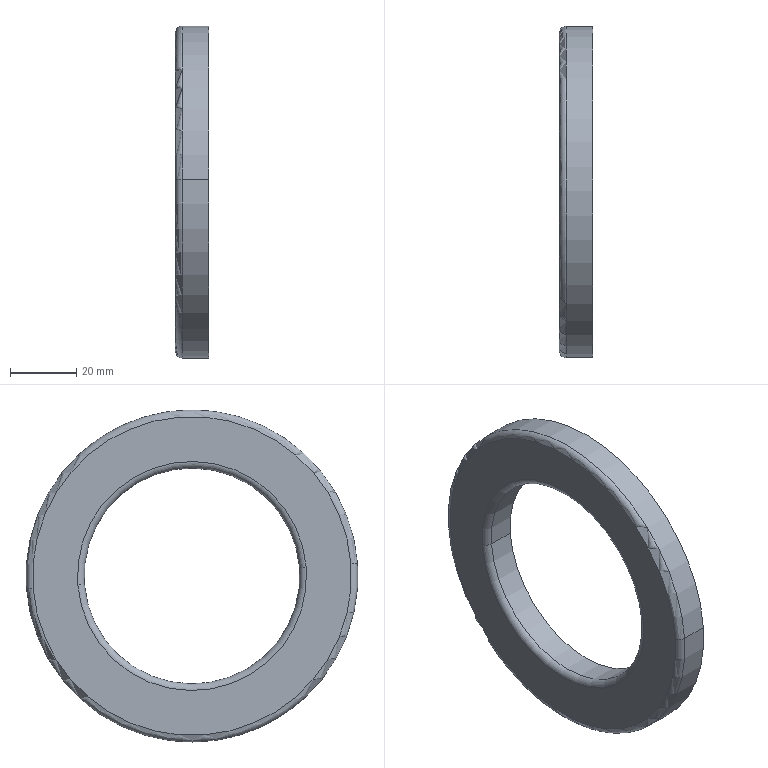Part | STEP file | Input 21 | 1 solid | 20 faces | box 10 x 100 x 100 mm | volume 8867 mm3 | cylinder 8 | torus 8 | plane 4 | commonest cylinder face diameters 65 x2 67 x2 98 x2 100 x2
STEP:
#1=CARTESIAN_POINT('',(0.,0.,0.));
#2=DIRECTION('',(0.,0.,1.));
#3=DIRECTION('',(1.,0.,0.));
#4=AXIS2_PLACEMENT_3D('',#1,#2,#3);
#5=CARTESIAN_POINT('',(-3648.,-33.401,2.578));
#6=VERTEX_POINT('',#5);
#7=CARTESIAN_POINT('',(-3648.,33.401,-2.578));
#8=VERTEX_POINT('',#7);
#9=CARTESIAN_POINT('',(-3648.,0.,0.));
#10=DIRECTION('',(1.,0.,0.));
#11=DIRECTION('',(0.,-0.997,0.07695));
#12=AXIS2_PLACEMENT_3D('',#9,#10,#11);
#13=CIRCLE('',#12,33.5);
#14=CARTESIAN_POINT('',(-3640.,0.,0.));
#15=DIRECTION('',(1.,0.,0.));
#16=DIRECTION('',(0.,-0.997,0.07695));
#17=AXIS2_PLACEMENT_3D('',#14,#15,#16);
#18=CYLINDRICAL_SURFACE('',#17,33.5);
#19=CARTESIAN_POINT('',(0.,-8.));
#20=DIRECTION('',(1.,0.));
#21=VECTOR('',#20,1.);
#22=LINE('',#19,#21);
#23=(GEOMETRIC_REPRESENTATION_CONTEXT(2)PARAMETRIC_REPRESENTATION_CONTEXT()REPRESENTATION_CONTEXT('',''));
#24=DEFINITIONAL_REPRESENTATION('',(#22),#23);
#25=PCURVE('',#18,#24);
#26=CARTESIAN_POINT('',(-3648.,0.,0.));
#27=DIRECTION('',(1.,0.,0.));
#28=DIRECTION('',(0.,-0.997,0.07695));
#29=AXIS2_PLACEMENT_3D('',#26,#27,#28);
#30=TOROIDAL_SURFACE('',#29,34.5,1.);
#31=CARTESIAN_POINT('',(0.,3.142));
#32=DIRECTION('',(1.,0.));
#33=VECTOR('',#32,1.);
#34=LINE('',#31,#33);
#35=(GEOMETRIC_REPRESENTATION_CONTEXT(2)PARAMETRIC_REPRESENTATION_CONTEXT()REPRESENTATION_CONTEXT('',''));
#36=DEFINITIONAL_REPRESENTATION('',(#34),#35);
#37=PCURVE('',#30,#36);
#38=SURFACE_CURVE('',#13,(#25,#37),.PCURVE_S1.);
#39=EDGE_CURVE('',#6,#8,#38,.T.);
#40=ORIENTED_EDGE('',*,*,#39,.T.);
#41=CARTESIAN_POINT('',(-3640.,33.401,-2.578));
#42=VERTEX_POINT('',#41);
#43=CARTESIAN_POINT('',(-3640.,33.401,-2.578));
#44=DIRECTION('',(1.,0.,0.));
#45=VECTOR('',#44,1.);
#46=LINE('',#43,#45);
#47=CARTESIAN_POINT('',(3.142,0.));
#48=DIRECTION('',(0.,1.));
#49=VECTOR('',#48,1.);
#50=LINE('',#47,#49);
#51=(GEOMETRIC_REPRESENTATION_CONTEXT(2)PARAMETRIC_REPRESENTATION_CONTEXT()REPRESENTATION_CONTEXT('',''));
#52=DEFINITIONAL_REPRESENTATION('',(#50),#51);
#53=PCURVE('',#18,#52);
#54=CARTESIAN_POINT('',(-3640.,0.,0.));
#55=DIRECTION('',(1.,0.,0.));
#56=DIRECTION('',(0.,-0.997,0.07695));
#57=AXIS2_PLACEMENT_3D('',#54,#55,#56);
#58=CYLINDRICAL_SURFACE('',#57,33.5);
#59=CARTESIAN_POINT('',(3.142,0.));
#60=DIRECTION('',(0.,1.));
#61=VECTOR('',#60,1.);
#62=LINE('',#59,#61);
#63=(GEOMETRIC_REPRESENTATION_CONTEXT(2)PARAMETRIC_REPRESENTATION_CONTEXT()REPRESENTATION_CONTEXT('',''));
#64=DEFINITIONAL_REPRESENTATION('',(#62),#63);
#65=PCURVE('',#58,#64);
#66=SURFACE_CURVE('',#46,(#53,#65),.PCURVE_S1.);
#67=EDGE_CURVE('',#8,#42,#66,.T.);
#68=ORIENTED_EDGE('',*,*,#67,.T.);
#69=CARTESIAN_POINT('',(-3640.,-33.401,2.578));
#70=VERTEX_POINT('',#69);
#71=CARTESIAN_POINT('',(-3640.,0.,0.));
#72=DIRECTION('',(1.,0.,0.));
#73=DIRECTION('',(0.,-0.997,0.07695));
#74=AXIS2_PLACEMENT_3D('',#71,#72,#73);
#75=CIRCLE('',#74,33.5);
#76=CARTESIAN_POINT('',(0.,0.));
#77=DIRECTION('',(1.,0.));
#78=VECTOR('',#77,1.);
#79=LINE('',#76,#78);
#80=(GEOMETRIC_REPRESENTATION_CONTEXT(2)PARAMETRIC_REPRESENTATION_CONTEXT()REPRESENTATION_CONTEXT('',''));
#81=DEFINITIONAL_REPRESENTATION('',(#79),#80);
#82=PCURVE('',#18,#81);
#83=CARTESIAN_POINT('',(-3640.,-33.401,2.578));
#84=DIRECTION('',(1.,0.,0.));
#85=DIRECTION('',(0.,-0.997,0.07695));
#86=AXIS2_PLACEMENT_3D('',#83,#84,#85);
#87=PLANE('',#86);
#88=CARTESIAN_POINT('',(-33.5,0.));
#89=DIRECTION('',(1.,0.));
#90=AXIS2_PLACEMENT_2D('',#88,#89);
#91=CIRCLE('',#90,33.5);
#92=(GEOMETRIC_REPRESENTATION_CONTEXT(2)PARAMETRIC_REPRESENTATION_CONTEXT()REPRESENTATION_CONTEXT('',''));
#93=DEFINITIONAL_REPRESENTATION('',(#91),#92);
#94=PCURVE('',#87,#93);
#95=SURFACE_CURVE('',#75,(#82,#94),.PCURVE_S1.);
#96=EDGE_CURVE('',#70,#42,#95,.T.);
#97=ORIENTED_EDGE('',*,*,#96,.F.);
#98=CARTESIAN_POINT('',(-3640.,-33.401,2.578));
#99=DIRECTION('',(1.,0.,0.));
#100=VECTOR('',#99,1.);
#101=LINE('',#98,#100);
#102=CARTESIAN_POINT('',(0.,0.));
#103=DIRECTION('',(0.,1.));
#104=VECTOR('',#103,1.);
#105=LINE('',#102,#104);
#106=(GEOMETRIC_REPRESENTATION_CONTEXT(2)PARAMETRIC_REPRESENTATION_CONTEXT()REPRESENTATION_CONTEXT('',''));
#107=DEFINITIONAL_REPRESENTATION('',(#105),#106);
#108=PCURVE('',#18,#107);
#109=CARTESIAN_POINT('',(6.283,0.));
#110=DIRECTION('',(0.,1.));
#111=VECTOR('',#110,1.);
#112=LINE('',#109,#111);
#113=(GEOMETRIC_REPRESENTATION_CONTEXT(2)PARAMETRIC_REPRESENTATION_CONTEXT()REPRESENTATION_CONTEXT('',''));
#114=DEFINITIONAL_REPRESENTATION('',(#112),#113);
#115=PCURVE('',#58,#114);
#116=SURFACE_CURVE('',#101,(#108,#115),.PCURVE_S1.);
#117=EDGE_CURVE('',#6,#70,#116,.T.);
#118=ORIENTED_EDGE('',*,*,#117,.F.);
#119=EDGE_LOOP('',(#40,#68,#97,#118));
#120=FACE_BOUND('',#119,.T.);
#121=ADVANCED_FACE('',(#120),#18,.T.);
#122=CARTESIAN_POINT('',(-3649.,-34.398,2.655));
#123=VERTEX_POINT('',#122);
#124=CARTESIAN_POINT('',(-3648.,-34.398,2.655));
#125=DIRECTION('',(0.,0.07695,0.997));
#126=DIRECTION('',(0.,-0.997,0.07695));
#127=AXIS2_PLACEMENT_3D('',#124,#125,#126);
#128=CIRCLE('',#127,1.);
#129=CARTESIAN_POINT('',(-3648.,0.,0.));
#130=DIRECTION('',(1.,0.,0.));
#131=DIRECTION('',(0.,-0.997,0.07695));
#132=AXIS2_PLACEMENT_3D('',#129,#130,#131);
#133=TOROIDAL_SURFACE('',#132,34.5,1.);
#134=CARTESIAN_POINT('',(6.283,0.));
#135=DIRECTION('',(0.,1.));
#136=VECTOR('',#135,1.);
#137=LINE('',#134,#136);
#138=(GEOMETRIC_REPRESENTATION_CONTEXT(2)PARAMETRIC_REPRESENTATION_CONTEXT()REPRESENTATION_CONTEXT('',''));
#139=DEFINITIONAL_REPRESENTATION('',(#137),#138);
#140=PCURVE('',#133,#139);
#141=CARTESIAN_POINT('',(0.,0.));
#142=DIRECTION('',(0.,1.));
#143=VECTOR('',#142,1.);
#144=LINE('',#141,#143);
#145=(GEOMETRIC_REPRESENTATION_CONTEXT(2)PARAMETRIC_REPRESENTATION_CONTEXT()REPRESENTATION_CONTEXT('',''));
#146=DEFINITIONAL_REPRESENTATION('',(#144),#145);
#147=PCURVE('',#30,#146);
#148=SURFACE_CURVE('',#128,(#140,#147),.PCURVE_S1.);
#149=EDGE_CURVE('',#6,#123,#148,.T.);
#150=ORIENTED_EDGE('',*,*,#149,.T.);
#151=CARTESIAN_POINT('',(-3649.,34.398,-2.655));
#152=VERTEX_POINT('',#151);
#153=CARTESIAN_POINT('',(-3649.,0.,0.));
#154=DIRECTION('',(1.,0.,0.));
#155=DIRECTION('',(0.,-0.997,0.07695));
#156=AXIS2_PLACEMENT_3D('',#153,#154,#155);
#157=CIRCLE('',#156,34.5);
#158=CARTESIAN_POINT('',(0.,4.712));
#159=DIRECTION('',(1.,0.));
#160=VECTOR('',#159,1.);
#161=LINE('',#158,#160);
#162=(GEOMETRIC_REPRESENTATION_CONTEXT(2)PARAMETRIC_REPRESENTATION_CONTEXT()REPRESENTATION_CONTEXT('',''));
#163=DEFINITIONAL_REPRESENTATION('',(#161),#162);
#164=PCURVE('',#133,#163);
#165=CARTESIAN_POINT('',(-3649.,-47.858,3.694));
#166=DIRECTION('',(1.,0.,0.));
#167=DIRECTION('',(0.,-0.997,0.07695));
#168=AXIS2_PLACEMENT_3D('',#165,#166,#167);
#169=PLANE('',#168);
#170=CARTESIAN_POINT('',(-48.,0.));
#171=DIRECTION('',(1.,0.));
#172=AXIS2_PLACEMENT_2D('',#170,#171);
#173=CIRCLE('',#172,34.5);
#174=(GEOMETRIC_REPRESENTATION_CONTEXT(2)PARAMETRIC_REPRESENTATION_CONTEXT()REPRESENTATION_CONTEXT('',''));
#175=DEFINITIONAL_REPRESENTATION('',(#173),#174);
#176=PCURVE('',#169,#175);
#177=SURFACE_CURVE('',#157,(#164,#176),.PCURVE_S1.);
#178=EDGE_CURVE('',#152,#123,#177,.T.);
#179=ORIENTED_EDGE('',*,*,#178,.F.);
#180=CARTESIAN_POINT('',(-3648.,34.398,-2.655));
#181=DIRECTION('',(0.,-0.07695,-0.997));
#182=DIRECTION('',(0.,0.997,-0.07695));
#183=AXIS2_PLACEMENT_3D('',#180,#181,#182);
#184=CIRCLE('',#183,1.);
#185=CARTESIAN_POINT('',(3.142,0.));
#186=DIRECTION('',(0.,1.));
#187=VECTOR('',#186,1.);
#188=LINE('',#185,#187);
#189=(GEOMETRIC_REPRESENTATION_CONTEXT(2)PARAMETRIC_REPRESENTATION_CONTEXT()REPRESENTATION_CONTEXT('',''));
#190=DEFINITIONAL_REPRESENTATION('',(#188),#189);
#191=PCURVE('',#133,#190);
#192=CARTESIAN_POINT('',(3.142,0.));
#193=DIRECTION('',(0.,1.));
#194=VECTOR('',#193,1.);
#195=LINE('',#192,#194);
#196=(GEOMETRIC_REPRESENTATION_CONTEXT(2)PARAMETRIC_REPRESENTATION_CONTEXT()REPRESENTATION_CONTEXT('',''));
#197=DEFINITIONAL_REPRESENTATION('',(#195),#196);
#198=PCURVE('',#30,#197);
#199=SURFACE_CURVE('',#184,(#191,#198),.PCURVE_S1.);
#200=EDGE_CURVE('',#8,#152,#199,.T.);
#201=ORIENTED_EDGE('',*,*,#200,.F.);
#202=CARTESIAN_POINT('',(-3648.,0.,0.));
#203=DIRECTION('',(1.,0.,0.));
#204=DIRECTION('',(0.,-0.997,0.07695));
#205=AXIS2_PLACEMENT_3D('',#202,#203,#204);
#206=CIRCLE('',#205,33.5);
#207=CARTESIAN_POINT('',(0.,3.142));
#208=DIRECTION('',(1.,0.));
#209=VECTOR('',#208,1.);
#210=LINE('',#207,#209);
#211=(GEOMETRIC_REPRESENTATION_CONTEXT(2)PARAMETRIC_REPRESENTATION_CONTEXT()REPRESENTATION_CONTEXT('',''));
#212=DEFINITIONAL_REPRESENTATION('',(#210),#211);
#213=PCURVE('',#133,#212);
#214=CARTESIAN_POINT('',(0.,-8.));
#215=DIRECTION('',(1.,0.));
#216=VECTOR('',#215,1.);
#217=LINE('',#214,#216);
#218=(GEOMETRIC_REPRESENTATION_CONTEXT(2)PARAMETRIC_REPRESENTATION_CONTEXT()REPRESENTATION_CONTEXT('',''));
#219=DEFINITIONAL_REPRESENTATION('',(#217),#218);
#220=PCURVE('',#58,#219);
#221=SURFACE_CURVE('',#206,(#213,#220),.PCURVE_S1.);
#222=EDGE_CURVE('',#8,#6,#221,.T.);
#223=ORIENTED_EDGE('',*,*,#222,.T.);
#224=EDGE_LOOP('',(#150,#179,#201,#223));
#225=FACE_BOUND('',#224,.F.);
#226=ADVANCED_FACE('',(#225),#133,.F.);
#227=CARTESIAN_POINT('',(-3649.,-47.858,3.694));
#228=VERTEX_POINT('',#227);
#229=CARTESIAN_POINT('',(-3648.,-48.855,3.771));
#230=VERTEX_POINT('',#229);
#231=CARTESIAN_POINT('',(-3648.,-47.858,3.694));
#232=DIRECTION('',(0.,0.07695,0.997));
#233=DIRECTION('',(0.,-0.997,0.07695));
#234=AXIS2_PLACEMENT_3D('',#231,#232,#233);
#235=CIRCLE('',#234,1.);
#236=CARTESIAN_POINT('',(-3648.,0.,0.));
#237=DIRECTION('',(1.,0.,0.));
#238=DIRECTION('',(0.,-0.997,0.07695));
#239=AXIS2_PLACEMENT_3D('',#236,#237,#238);
#240=TOROIDAL_SURFACE('',#239,48.,1.);
#241=CARTESIAN_POINT('',(6.283,0.));
#242=DIRECTION('',(0.,1.));
#243=VECTOR('',#242,1.);
#244=LINE('',#241,#243);
#245=(GEOMETRIC_REPRESENTATION_CONTEXT(2)PARAMETRIC_REPRESENTATION_CONTEXT()REPRESENTATION_CONTEXT('',''));
#246=DEFINITIONAL_REPRESENTATION('',(#244),#245);
#247=PCURVE('',#240,#246);
#248=CARTESIAN_POINT('',(-3648.,0.,0.));
#249=DIRECTION('',(1.,0.,0.));
#250=DIRECTION('',(0.,-0.997,0.07695));
#251=AXIS2_PLACEMENT_3D('',#248,#249,#250);
#252=TOROIDAL_SURFACE('',#251,48.,1.);
#253=CARTESIAN_POINT('',(0.,0.));
#254=DIRECTION('',(0.,1.));
#255=VECTOR('',#254,1.);
#256=LINE('',#253,#255);
#257=(GEOMETRIC_REPRESENTATION_CONTEXT(2)PARAMETRIC_REPRESENTATION_CONTEXT()REPRESENTATION_CONTEXT('',''));
#258=DEFINITIONAL_REPRESENTATION('',(#256),#257);
#259=PCURVE('',#252,#258);
#260=SURFACE_CURVE('',#235,(#247,#259),.PCURVE_S1.);
#261=EDGE_CURVE('',#228,#230,#260,.T.);
#262=ORIENTED_EDGE('',*,*,#261,.T.);
#263=CARTESIAN_POINT('',(-3648.,48.855,-3.771));
#264=VERTEX_POINT('',#263);
#265=CARTESIAN_POINT('',(-3648.,0.,0.));
#266=DIRECTION('',(1.,0.,0.));
#267=DIRECTION('',(0.,-0.997,0.07695));
#268=AXIS2_PLACEMENT_3D('',#265,#266,#267);
#269=CIRCLE('',#268,49.);
#270=CARTESIAN_POINT('',(0.,6.283));
#271=DIRECTION('',(1.,0.));
#272=VECTOR('',#271,1.);
#273=LINE('',#270,#272);
#274=(GEOMETRIC_REPRESENTATION_CONTEXT(2)PARAMETRIC_REPRESENTATION_CONTEXT()REPRESENTATION_CONTEXT('',''));
#275=DEFINITIONAL_REPRESENTATION('',(#273),#274);
#276=PCURVE('',#240,#275);
#277=CARTESIAN_POINT('',(-3640.,0.,0.));
#278=DIRECTION('',(1.,0.,0.));
#279=DIRECTION('',(0.,-0.997,0.07695));
#280=AXIS2_PLACEMENT_3D('',#277,#278,#279);
#281=CYLINDRICAL_SURFACE('',#280,49.);
#282=CARTESIAN_POINT('',(0.,-8.));
#283=DIRECTION('',(1.,0.));
#284=VECTOR('',#283,1.);
#285=LINE('',#282,#284);
#286=(GEOMETRIC_REPRESENTATION_CONTEXT(2)PARAMETRIC_REPRESENTATION_CONTEXT()REPRESENTATION_CONTEXT('',''));
#287=DEFINITIONAL_REPRESENTATION('',(#285),#286);
#288=PCURVE('',#281,#287);
#289=SURFACE_CURVE('',#269,(#276,#288),.PCURVE_S1.);
#290=EDGE_CURVE('',#264,#230,#289,.T.);
#291=ORIENTED_EDGE('',*,*,#290,.F.);
#292=CARTESIAN_POINT('',(-3649.,47.858,-3.694));
#293=VERTEX_POINT('',#292);
#294=CARTESIAN_POINT('',(-3648.,47.858,-3.694));
#295=DIRECTION('',(0.,-0.07695,-0.997));
#296=DIRECTION('',(0.,0.997,-0.07695));
#297=AXIS2_PLACEMENT_3D('',#294,#295,#296);
#298=CIRCLE('',#297,1.);
#299=CARTESIAN_POINT('',(3.142,0.));
#300=DIRECTION('',(0.,1.));
#301=VECTOR('',#300,1.);
#302=LINE('',#299,#301);
#303=(GEOMETRIC_REPRESENTATION_CONTEXT(2)PARAMETRIC_REPRESENTATION_CONTEXT()REPRESENTATION_CONTEXT('',''));
#304=DEFINITIONAL_REPRESENTATION('',(#302),#303);
#305=PCURVE('',#240,#304);
#306=CARTESIAN_POINT('',(3.142,0.));
#307=DIRECTION('',(0.,1.));
#308=VECTOR('',#307,1.);
#309=LINE('',#306,#308);
#310=(GEOMETRIC_REPRESENTATION_CONTEXT(2)PARAMETRIC_REPRESENTATION_CONTEXT()REPRESENTATION_CONTEXT('',''));
#311=DEFINITIONAL_REPRESENTATION('',(#309),#310);
#312=PCURVE('',#252,#311);
#313=SURFACE_CURVE('',#298,(#305,#312),.PCURVE_S1.);
#314=EDGE_CURVE('',#293,#264,#313,.T.);
#315=ORIENTED_EDGE('',*,*,#314,.F.);
#316=CARTESIAN_POINT('',(-3649.,0.,0.));
#317=DIRECTION('',(1.,0.,0.));
#318=DIRECTION('',(0.,-0.997,0.07695));
#319=AXIS2_PLACEMENT_3D('',#316,#317,#318);
#320=CIRCLE('',#319,48.);
#321=CARTESIAN_POINT('',(0.,4.712));
#322=DIRECTION('',(1.,0.));
#323=VECTOR('',#322,1.);
#324=LINE('',#321,#323);
#325=(GEOMETRIC_REPRESENTATION_CONTEXT(2)PARAMETRIC_REPRESENTATION_CONTEXT()REPRESENTATION_CONTEXT('',''));
#326=DEFINITIONAL_REPRESENTATION('',(#324),#325);
#327=PCURVE('',#240,#326);
#328=CARTESIAN_POINT('',(-48.,0.));
#329=DIRECTION('',(1.,0.));
#330=AXIS2_PLACEMENT_2D('',#328,#329);
#331=CIRCLE('',#330,48.);
#332=(GEOMETRIC_REPRESENTATION_CONTEXT(2)PARAMETRIC_REPRESENTATION_CONTEXT()REPRESENTATION_CONTEXT('',''));
#333=DEFINITIONAL_REPRESENTATION('',(#331),#332);
#334=PCURVE('',#169,#333);
#335=SURFACE_CURVE('',#320,(#327,#334),.PCURVE_S1.);
#336=EDGE_CURVE('',#293,#228,#335,.T.);
#337=ORIENTED_EDGE('',*,*,#336,.T.);
#338=EDGE_LOOP('',(#262,#291,#315,#337));
#339=FACE_BOUND('',#338,.F.);
#340=ADVANCED_FACE('',(#339),#240,.F.);
#341=CARTESIAN_POINT('',(-3640.,-48.855,3.771));
#342=VERTEX_POINT('',#341);
#343=CARTESIAN_POINT('',(-3640.,-48.855,3.771));
#344=DIRECTION('',(1.,0.,0.));
#345=VECTOR('',#344,1.);
#346=LINE('',#343,#345);
#347=CARTESIAN_POINT('',(6.283,0.));
#348=DIRECTION('',(0.,1.));
#349=VECTOR('',#348,1.);
#350=LINE('',#347,#349);
#351=(GEOMETRIC_REPRESENTATION_CONTEXT(2)PARAMETRIC_REPRESENTATION_CONTEXT()REPRESENTATION_CONTEXT('',''));
#352=DEFINITIONAL_REPRESENTATION('',(#350),#351);
#353=PCURVE('',#281,#352);
#354=CARTESIAN_POINT('',(-3640.,0.,0.));
#355=DIRECTION('',(1.,0.,0.));
#356=DIRECTION('',(0.,-0.997,0.07695));
#357=AXIS2_PLACEMENT_3D('',#354,#355,#356);
#358=CYLINDRICAL_SURFACE('',#357,49.);
#359=CARTESIAN_POINT('',(0.,0.));
#360=DIRECTION('',(0.,1.));
#361=VECTOR('',#360,1.);
#362=LINE('',#359,#361);
#363=(GEOMETRIC_REPRESENTATION_CONTEXT(2)PARAMETRIC_REPRESENTATION_CONTEXT()REPRESENTATION_CONTEXT('',''));
#364=DEFINITIONAL_REPRESENTATION('',(#362),#363);
#365=PCURVE('',#358,#364);
#366=SURFACE_CURVE('',#346,(#353,#365),.PCURVE_S1.);
#367=EDGE_CURVE('',#230,#342,#366,.T.);
#368=ORIENTED_EDGE('',*,*,#367,.T.);
#369=CARTESIAN_POINT('',(-3640.,48.855,-3.771));
#370=VERTEX_POINT('',#369);
#371=CARTESIAN_POINT('',(-3640.,0.,0.));
#372=DIRECTION('',(1.,0.,0.));
#373=DIRECTION('',(0.,-0.997,0.07695));
#374=AXIS2_PLACEMENT_3D('',#371,#372,#373);
#375=CIRCLE('',#374,49.);
#376=CARTESIAN_POINT('',(0.,0.));
#377=DIRECTION('',(1.,0.));
#378=VECTOR('',#377,1.);
#379=LINE('',#376,#378);
#380=(GEOMETRIC_REPRESENTATION_CONTEXT(2)PARAMETRIC_REPRESENTATION_CONTEXT()REPRESENTATION_CONTEXT('',''));
#381=DEFINITIONAL_REPRESENTATION('',(#379),#380);
#382=PCURVE('',#281,#381);
#383=CARTESIAN_POINT('',(-3640.,-49.852,3.848));
#384=DIRECTION('',(1.,0.,0.));
#385=DIRECTION('',(0.,-0.997,0.07695));
#386=AXIS2_PLACEMENT_3D('',#383,#384,#385);
#387=PLANE('',#386);
#388=CARTESIAN_POINT('',(-50.,0.));
#389=DIRECTION('',(1.,0.));
#390=AXIS2_PLACEMENT_2D('',#388,#389);
#391=CIRCLE('',#390,49.);
#392=(GEOMETRIC_REPRESENTATION_CONTEXT(2)PARAMETRIC_REPRESENTATION_CONTEXT()REPRESENTATION_CONTEXT('',''));
#393=DEFINITIONAL_REPRESENTATION('',(#391),#392);
#394=PCURVE('',#387,#393);
#395=SURFACE_CURVE('',#375,(#382,#394),.PCURVE_S1.);
#396=EDGE_CURVE('',#370,#342,#395,.T.);
#397=ORIENTED_EDGE('',*,*,#396,.F.);
#398=CARTESIAN_POINT('',(-3640.,48.855,-3.771));
#399=DIRECTION('',(1.,0.,0.));
#400=VECTOR('',#399,1.);
#401=LINE('',#398,#400);
#402=CARTESIAN_POINT('',(3.142,0.));
#403=DIRECTION('',(0.,1.));
#404=VECTOR('',#403,1.);
#405=LINE('',#402,#404);
#406=(GEOMETRIC_REPRESENTATION_CONTEXT(2)PARAMETRIC_REPRESENTATION_CONTEXT()REPRESENTATION_CONTEXT('',''));
#407=DEFINITIONAL_REPRESENTATION('',(#405),#406);
#408=PCURVE('',#281,#407);
#409=CARTESIAN_POINT('',(3.142,0.));
#410=DIRECTION('',(0.,1.));
#411=VECTOR('',#410,1.);
#412=LINE('',#409,#411);
#413=(GEOMETRIC_REPRESENTATION_CONTEXT(2)PARAMETRIC_REPRESENTATION_CONTEXT()REPRESENTATION_CONTEXT('',''));
#414=DEFINITIONAL_REPRESENTATION('',(#412),#413);
#415=PCURVE('',#358,#414);
#416=SURFACE_CURVE('',#401,(#408,#415),.PCURVE_S1.);
#417=EDGE_CURVE('',#264,#370,#416,.T.);
#418=ORIENTED_EDGE('',*,*,#417,.F.);
#419=ORIENTED_EDGE('',*,*,#290,.T.);
#420=EDGE_LOOP('',(#368,#397,#418,#419));
#421=FACE_BOUND('',#420,.F.);
#422=ADVANCED_FACE('',(#421),#281,.F.);
#423=CARTESIAN_POINT('',(-3648.,-49.852,3.848));
#424=VERTEX_POINT('',#423);
#425=CARTESIAN_POINT('',(-3648.,49.852,-3.848));
#426=VERTEX_POINT('',#425);
#427=CARTESIAN_POINT('',(-3648.,0.,0.));
#428=DIRECTION('',(1.,0.,0.));
#429=DIRECTION('',(0.,-0.997,0.07695));
#430=AXIS2_PLACEMENT_3D('',#427,#428,#429);
#431=CIRCLE('',#430,50.);
#432=CARTESIAN_POINT('',(-3640.,0.,0.));
#433=DIRECTION('',(1.,0.,0.));
#434=DIRECTION('',(0.,-0.997,0.07695));
#435=AXIS2_PLACEMENT_3D('',#432,#433,#434);
#436=CYLINDRICAL_SURFACE('',#435,50.);
#437=CARTESIAN_POINT('',(0.,-8.));
#438=DIRECTION('',(1.,0.));
#439=VECTOR('',#438,1.);
#440=LINE('',#437,#439);
#441=(GEOMETRIC_REPRESENTATION_CONTEXT(2)PARAMETRIC_REPRESENTATION_CONTEXT()REPRESENTATION_CONTEXT('',''));
#442=DEFINITIONAL_REPRESENTATION('',(#440),#441);
#443=PCURVE('',#436,#442);
#444=CARTESIAN_POINT('',(-3648.,0.,0.));
#445=DIRECTION('',(1.,0.,0.));
#446=DIRECTION('',(0.,-0.997,0.07695));
#447=AXIS2_PLACEMENT_3D('',#444,#445,#446);
#448=TOROIDAL_SURFACE('',#447,48.,2.);
#449=CARTESIAN_POINT('',(0.,6.283));
#450=DIRECTION('',(1.,0.));
#451=VECTOR('',#450,1.);
#452=LINE('',#449,#451);
#453=(GEOMETRIC_REPRESENTATION_CONTEXT(2)PARAMETRIC_REPRESENTATION_CONTEXT()REPRESENTATION_CONTEXT('',''));
#454=DEFINITIONAL_REPRESENTATION('',(#452),#453);
#455=PCURVE('',#448,#454);
#456=SURFACE_CURVE('',#431,(#443,#455),.PCURVE_S1.);
#457=EDGE_CURVE('',#424,#426,#456,.T.);
#458=ORIENTED_EDGE('',*,*,#457,.T.);
#459=CARTESIAN_POINT('',(-3640.,49.852,-3.848));
#460=VERTEX_POINT('',#459);
#461=CARTESIAN_POINT('',(-3640.,49.852,-3.848));
#462=DIRECTION('',(1.,0.,0.));
#463=VECTOR('',#462,1.);
#464=LINE('',#461,#463);
#465=CARTESIAN_POINT('',(3.142,0.));
#466=DIRECTION('',(0.,1.));
#467=VECTOR('',#466,1.);
#468=LINE('',#465,#467);
#469=(GEOMETRIC_REPRESENTATION_CONTEXT(2)PARAMETRIC_REPRESENTATION_CONTEXT()REPRESENTATION_CONTEXT('',''));
#470=DEFINITIONAL_REPRESENTATION('',(#468),#469);
#471=PCURVE('',#436,#470);
#472=CARTESIAN_POINT('',(-3640.,0.,0.));
#473=DIRECTION('',(1.,0.,0.));
#474=DIRECTION('',(0.,-0.997,0.07695));
#475=AXIS2_PLACEMENT_3D('',#472,#473,#474);
#476=CYLINDRICAL_SURFACE('',#475,50.);
#477=CARTESIAN_POINT('',(3.142,0.));
#478=DIRECTION('',(0.,1.));
#479=VECTOR('',#478,1.);
#480=LINE('',#477,#479);
#481=(GEOMETRIC_REPRESENTATION_CONTEXT(2)PARAMETRIC_REPRESENTATION_CONTEXT()REPRESENTATION_CONTEXT('',''));
#482=DEFINITIONAL_REPRESENTATION('',(#480),#481);
#483=PCURVE('',#476,#482);
#484=SURFACE_CURVE('',#464,(#471,#483),.PCURVE_S1.);
#485=EDGE_CURVE('',#426,#460,#484,.T.);
#486=ORIENTED_EDGE('',*,*,#485,.T.);
#487=CARTESIAN_POINT('',(-3640.,-49.852,3.848));
#488=VERTEX_POINT('',#487);
#489=CARTESIAN_POINT('',(-3640.,0.,0.));
#490=DIRECTION('',(1.,0.,0.));
#491=DIRECTION('',(0.,-0.997,0.07695));
#492=AXIS2_PLACEMENT_3D('',#489,#490,#491);
#493=CIRCLE('',#492,50.);
#494=CARTESIAN_POINT('',(0.,0.));
#495=DIRECTION('',(1.,0.));
#496=VECTOR('',#495,1.);
#497=LINE('',#494,#496);
#498=(GEOMETRIC_REPRESENTATION_CONTEXT(2)PARAMETRIC_REPRESENTATION_CONTEXT()REPRESENTATION_CONTEXT('',''));
#499=DEFINITIONAL_REPRESENTATION('',(#497),#498);
#500=PCURVE('',#436,#499);
#501=CARTESIAN_POINT('',(-50.,0.));
#502=DIRECTION('',(1.,0.));
#503=AXIS2_PLACEMENT_2D('',#501,#502);
#504=CIRCLE('',#503,50.);
#505=(GEOMETRIC_REPRESENTATION_CONTEXT(2)PARAMETRIC_REPRESENTATION_CONTEXT()REPRESENTATION_CONTEXT('',''));
#506=DEFINITIONAL_REPRESENTATION('',(#504),#505);
#507=PCURVE('',#387,#506);
#508=SURFACE_CURVE('',#493,(#500,#507),.PCURVE_S1.);
#509=EDGE_CURVE('',#488,#460,#508,.T.);
#510=ORIENTED_EDGE('',*,*,#509,.F.);
#511=CARTESIAN_POINT('',(-3640.,-49.852,3.848));
#512=DIRECTION('',(1.,0.,0.));
#513=VECTOR('',#512,1.);
#514=LINE('',#511,#513);
#515=CARTESIAN_POINT('',(0.,0.));
#516=DIRECTION('',(0.,1.));
#517=VECTOR('',#516,1.);
#518=LINE('',#515,#517);
#519=(GEOMETRIC_REPRESENTATION_CONTEXT(2)PARAMETRIC_REPRESENTATION_CONTEXT()REPRESENTATION_CONTEXT('',''));
#520=DEFINITIONAL_REPRESENTATION('',(#518),#519);
#521=PCURVE('',#436,#520);
#522=CARTESIAN_POINT('',(6.283,0.));
#523=DIRECTION('',(0.,1.));
#524=VECTOR('',#523,1.);
#525=LINE('',#522,#524);
#526=(GEOMETRIC_REPRESENTATION_CONTEXT(2)PARAMETRIC_REPRESENTATION_CONTEXT()REPRESENTATION_CONTEXT('',''));
#527=DEFINITIONAL_REPRESENTATION('',(#525),#526);
#528=PCURVE('',#476,#527);
#529=SURFACE_CURVE('',#514,(#521,#528),.PCURVE_S1.);
#530=EDGE_CURVE('',#424,#488,#529,.T.);
#531=ORIENTED_EDGE('',*,*,#530,.F.);
#532=EDGE_LOOP('',(#458,#486,#510,#531));
#533=FACE_BOUND('',#532,.T.);
#534=ADVANCED_FACE('',(#533),#436,.T.);
#535=CARTESIAN_POINT('',(-3650.,-47.858,3.694));
#536=VERTEX_POINT('',#535);
#537=CARTESIAN_POINT('',(-3650.,47.858,-3.694));
#538=VERTEX_POINT('',#537);
#539=CARTESIAN_POINT('',(-3650.,0.,0.));
#540=DIRECTION('',(1.,0.,0.));
#541=DIRECTION('',(0.,-0.997,0.07695));
#542=AXIS2_PLACEMENT_3D('',#539,#540,#541);
#543=CIRCLE('',#542,48.);
#544=CARTESIAN_POINT('',(0.,4.712));
#545=DIRECTION('',(1.,0.));
#546=VECTOR('',#545,1.);
#547=LINE('',#544,#546);
#548=(GEOMETRIC_REPRESENTATION_CONTEXT(2)PARAMETRIC_REPRESENTATION_CONTEXT()REPRESENTATION_CONTEXT('',''));
#549=DEFINITIONAL_REPRESENTATION('',(#547),#548);
#550=PCURVE('',#448,#549);
#551=CARTESIAN_POINT('',(-3650.,-34.398,2.655));
#552=DIRECTION('',(-1.,0.,0.));
#553=DIRECTION('',(0.,0.997,-0.07695));
#554=AXIS2_PLACEMENT_3D('',#551,#552,#553);
#555=PLANE('',#554);
#556=CARTESIAN_POINT('',(-13.5,0.));
#557=CARTESIAN_POINT('',(-13.5,83.138));
#558=CARTESIAN_POINT('',(58.5,41.569));
#559=CARTESIAN_POINT('',(130.5,0.));
#560=CARTESIAN_POINT('',(58.5,-41.569));
#561=CARTESIAN_POINT('',(-13.5,-83.138));
#562=CARTESIAN_POINT('',(-13.5,0.));
#563=(BOUNDED_CURVE()B_SPLINE_CURVE(2,(#556,#557,#558,#559,#560,#561,#562),.UNSPECIFIED.,.T.,.F.)B_SPLINE_CURVE_WITH_KNOTS((1,2,2,2,2,1),(-2.094,0.,2.094,4.189,6.283,8.378),.UNSPECIFIED.)CURVE()GEOMETRIC_REPRESENTATION_ITEM()RATIONAL_B_SPLINE_CURVE((1.,0.5,1.,0.5,1.,0.5,1.))REPRESENTATION_ITEM(''));
#564=(GEOMETRIC_REPRESENTATION_CONTEXT(2)PARAMETRIC_REPRESENTATION_CONTEXT()REPRESENTATION_CONTEXT('',''));
#565=DEFINITIONAL_REPRESENTATION('',(#563),#564);
#566=PCURVE('',#555,#565);
#567=SURFACE_CURVE('',#543,(#550,#566),.PCURVE_S1.);
#568=EDGE_CURVE('',#536,#538,#567,.T.);
#569=ORIENTED_EDGE('',*,*,#568,.T.);
#570=CARTESIAN_POINT('',(-3648.,47.858,-3.694));
#571=DIRECTION('',(0.,-0.07695,-0.997));
#572=DIRECTION('',(0.,0.997,-0.07695));
#573=AXIS2_PLACEMENT_3D('',#570,#571,#572);
#574=CIRCLE('',#573,2.);
#575=CARTESIAN_POINT('',(3.142,0.));
#576=DIRECTION('',(0.,1.));
#577=VECTOR('',#576,1.);
#578=LINE('',#575,#577);
#579=(GEOMETRIC_REPRESENTATION_CONTEXT(2)PARAMETRIC_REPRESENTATION_CONTEXT()REPRESENTATION_CONTEXT('',''));
#580=DEFINITIONAL_REPRESENTATION('',(#578),#579);
#581=PCURVE('',#448,#580);
#582=CARTESIAN_POINT('',(-3648.,0.,0.));
#583=DIRECTION('',(1.,0.,0.));
#584=DIRECTION('',(0.,-0.997,0.07695));
#585=AXIS2_PLACEMENT_3D('',#582,#583,#584);
#586=TOROIDAL_SURFACE('',#585,48.,2.);
#587=CARTESIAN_POINT('',(3.142,0.));
#588=DIRECTION('',(0.,1.));
#589=VECTOR('',#588,1.);
#590=LINE('',#587,#589);
#591=(GEOMETRIC_REPRESENTATION_CONTEXT(2)PARAMETRIC_REPRESENTATION_CONTEXT()REPRESENTATION_CONTEXT('',''));
#592=DEFINITIONAL_REPRESENTATION('',(#590),#591);
#593=PCURVE('',#586,#592);
#594=SURFACE_CURVE('',#574,(#581,#593),.PCURVE_S1.);
#595=EDGE_CURVE('',#538,#426,#594,.T.);
#596=ORIENTED_EDGE('',*,*,#595,.T.);
#597=ORIENTED_EDGE('',*,*,#457,.F.);
#598=CARTESIAN_POINT('',(-3648.,-47.858,3.694));
#599=DIRECTION('',(0.,0.07695,0.997));
#600=DIRECTION('',(0.,-0.997,0.07695));
#601=AXIS2_PLACEMENT_3D('',#598,#599,#600);
#602=CIRCLE('',#601,2.);
#603=CARTESIAN_POINT('',(0.,0.));
#604=DIRECTION('',(0.,1.));
#605=VECTOR('',#604,1.);
#606=LINE('',#603,#605);
#607=(GEOMETRIC_REPRESENTATION_CONTEXT(2)PARAMETRIC_REPRESENTATION_CONTEXT()REPRESENTATION_CONTEXT('',''));
#608=DEFINITIONAL_REPRESENTATION('',(#606),#607);
#609=PCURVE('',#448,#608);
#610=CARTESIAN_POINT('',(6.283,0.));
#611=DIRECTION('',(0.,1.));
#612=VECTOR('',#611,1.);
#613=LINE('',#610,#612);
#614=(GEOMETRIC_REPRESENTATION_CONTEXT(2)PARAMETRIC_REPRESENTATION_CONTEXT()REPRESENTATION_CONTEXT('',''));
#615=DEFINITIONAL_REPRESENTATION('',(#613),#614);
#616=PCURVE('',#586,#615);
#617=SURFACE_CURVE('',#602,(#609,#616),.PCURVE_S1.);
#618=EDGE_CURVE('',#536,#424,#617,.T.);
#619=ORIENTED_EDGE('',*,*,#618,.F.);
#620=EDGE_LOOP('',(#569,#596,#597,#619));
#621=FACE_BOUND('',#620,.T.);
#622=ADVANCED_FACE('',(#621),#448,.T.);
#623=CARTESIAN_POINT('',(-3648.,-32.404,2.501));
#624=VERTEX_POINT('',#623);
#625=CARTESIAN_POINT('',(-3648.,32.404,-2.501));
#626=VERTEX_POINT('',#625);
#627=CARTESIAN_POINT('',(-3648.,0.,0.));
#628=DIRECTION('',(1.,0.,0.));
#629=DIRECTION('',(0.,-0.997,0.07695));
#630=AXIS2_PLACEMENT_3D('',#627,#628,#629);
#631=CIRCLE('',#630,32.5);
#632=CARTESIAN_POINT('',(-3648.,0.,0.));
#633=DIRECTION('',(1.,0.,0.));
#634=DIRECTION('',(0.,-0.997,0.07695));
#635=AXIS2_PLACEMENT_3D('',#632,#633,#634);
#636=TOROIDAL_SURFACE('',#635,34.5,2.);
#637=CARTESIAN_POINT('',(0.,3.142));
#638=DIRECTION('',(1.,0.));
#639=VECTOR('',#638,1.);
#640=LINE('',#637,#639);
#641=(GEOMETRIC_REPRESENTATION_CONTEXT(2)PARAMETRIC_REPRESENTATION_CONTEXT()REPRESENTATION_CONTEXT('',''));
#642=DEFINITIONAL_REPRESENTATION('',(#640),#641);
#643=PCURVE('',#636,#642);
#644=CARTESIAN_POINT('',(-3640.,0.,0.));
#645=DIRECTION('',(1.,0.,0.));
#646=DIRECTION('',(0.,-0.997,0.07695));
#647=AXIS2_PLACEMENT_3D('',#644,#645,#646);
#648=CYLINDRICAL_SURFACE('',#647,32.5);
#649=CARTESIAN_POINT('',(0.,-8.));
#650=DIRECTION('',(1.,0.));
#651=VECTOR('',#650,1.);
#652=LINE('',#649,#651);
#653=(GEOMETRIC_REPRESENTATION_CONTEXT(2)PARAMETRIC_REPRESENTATION_CONTEXT()REPRESENTATION_CONTEXT('',''));
#654=DEFINITIONAL_REPRESENTATION('',(#652),#653);
#655=PCURVE('',#648,#654);
#656=SURFACE_CURVE('',#631,(#643,#655),.PCURVE_S1.);
#657=EDGE_CURVE('',#624,#626,#656,.T.);
#658=ORIENTED_EDGE('',*,*,#657,.T.);
#659=CARTESIAN_POINT('',(-3650.,34.398,-2.655));
#660=VERTEX_POINT('',#659);
#661=CARTESIAN_POINT('',(-3648.,34.398,-2.655));
#662=DIRECTION('',(0.,-0.07695,-0.997));
#663=DIRECTION('',(0.,0.997,-0.07695));
#664=AXIS2_PLACEMENT_3D('',#661,#662,#663);
#665=CIRCLE('',#664,2.);
#666=CARTESIAN_POINT('',(3.142,0.));
#667=DIRECTION('',(0.,1.));
#668=VECTOR('',#667,1.);
#669=LINE('',#666,#668);
#670=(GEOMETRIC_REPRESENTATION_CONTEXT(2)PARAMETRIC_REPRESENTATION_CONTEXT()REPRESENTATION_CONTEXT('',''));
#671=DEFINITIONAL_REPRESENTATION('',(#669),#670);
#672=PCURVE('',#636,#671);
#673=CARTESIAN_POINT('',(-3648.,0.,0.));
#674=DIRECTION('',(1.,0.,0.));
#675=DIRECTION('',(0.,-0.997,0.07695));
#676=AXIS2_PLACEMENT_3D('',#673,#674,#675);
#677=TOROIDAL_SURFACE('',#676,34.5,2.);
#678=CARTESIAN_POINT('',(3.142,0.));
#679=DIRECTION('',(0.,1.));
#680=VECTOR('',#679,1.);
#681=LINE('',#678,#680);
#682=(GEOMETRIC_REPRESENTATION_CONTEXT(2)PARAMETRIC_REPRESENTATION_CONTEXT()REPRESENTATION_CONTEXT('',''));
#683=DEFINITIONAL_REPRESENTATION('',(#681),#682);
#684=PCURVE('',#677,#683);
#685=SURFACE_CURVE('',#665,(#672,#684),.PCURVE_S1.);
#686=EDGE_CURVE('',#626,#660,#685,.T.);
#687=ORIENTED_EDGE('',*,*,#686,.T.);
#688=CARTESIAN_POINT('',(-3650.,-34.398,2.655));
#689=VERTEX_POINT('',#688);
#690=CARTESIAN_POINT('',(-3650.,0.,0.));
#691=DIRECTION('',(1.,0.,0.));
#692=DIRECTION('',(0.,-0.997,0.07695));
#693=AXIS2_PLACEMENT_3D('',#690,#691,#692);
#694=CIRCLE('',#693,34.5);
#695=CARTESIAN_POINT('',(0.,4.712));
#696=DIRECTION('',(1.,0.));
#697=VECTOR('',#696,1.);
#698=LINE('',#695,#697);
#699=(GEOMETRIC_REPRESENTATION_CONTEXT(2)PARAMETRIC_REPRESENTATION_CONTEXT()REPRESENTATION_CONTEXT('',''));
#700=DEFINITIONAL_REPRESENTATION('',(#698),#699);
#701=PCURVE('',#636,#700);
#702=CARTESIAN_POINT('',(0.,0.));
#703=CARTESIAN_POINT('',(0.,59.756));
#704=CARTESIAN_POINT('',(51.75,29.878));
#705=CARTESIAN_POINT('',(103.5,0.));
#706=CARTESIAN_POINT('',(51.75,-29.878));
#707=CARTESIAN_POINT('',(0.,-59.756));
#708=CARTESIAN_POINT('',(0.,0.));
#709=(BOUNDED_CURVE()B_SPLINE_CURVE(2,(#702,#703,#704,#705,#706,#707,#708),.UNSPECIFIED.,.T.,.F.)B_SPLINE_CURVE_WITH_KNOTS((1,2,2,2,2,1),(-2.094,0.,2.094,4.189,6.283,8.378),.UNSPECIFIED.)CURVE()GEOMETRIC_REPRESENTATION_ITEM()RATIONAL_B_SPLINE_CURVE((1.,0.5,1.,0.5,1.,0.5,1.))REPRESENTATION_ITEM(''));
#710=(GEOMETRIC_REPRESENTATION_CONTEXT(2)PARAMETRIC_REPRESENTATION_CONTEXT()REPRESENTATION_CONTEXT('',''));
#711=DEFINITIONAL_REPRESENTATION('',(#709),#710);
#712=PCURVE('',#555,#711);
#713=SURFACE_CURVE('',#694,(#701,#712),.PCURVE_S1.);
#714=EDGE_CURVE('',#689,#660,#713,.T.);
#715=ORIENTED_EDGE('',*,*,#714,.F.);
#716=CARTESIAN_POINT('',(-3648.,-34.398,2.655));
#717=DIRECTION('',(0.,0.07695,0.997));
#718=DIRECTION('',(0.,-0.997,0.07695));
#719=AXIS2_PLACEMENT_3D('',#716,#717,#718);
#720=CIRCLE('',#719,2.);
#721=CARTESIAN_POINT('',(0.,0.));
#722=DIRECTION('',(0.,1.));
#723=VECTOR('',#722,1.);
#724=LINE('',#721,#723);
#725=(GEOMETRIC_REPRESENTATION_CONTEXT(2)PARAMETRIC_REPRESENTATION_CONTEXT()REPRESENTATION_CONTEXT('',''));
#726=DEFINITIONAL_REPRESENTATION('',(#724),#725);
#727=PCURVE('',#636,#726);
#728=CARTESIAN_POINT('',(6.283,0.));
#729=DIRECTION('',(0.,1.));
#730=VECTOR('',#729,1.);
#731=LINE('',#728,#730);
#732=(GEOMETRIC_REPRESENTATION_CONTEXT(2)PARAMETRIC_REPRESENTATION_CONTEXT()REPRESENTATION_CONTEXT('',''));
#733=DEFINITIONAL_REPRESENTATION('',(#731),#732);
#734=PCURVE('',#677,#733);
#735=SURFACE_CURVE('',#720,(#727,#734),.PCURVE_S1.);
#736=EDGE_CURVE('',#624,#689,#735,.T.);
#737=ORIENTED_EDGE('',*,*,#736,.F.);
#738=EDGE_LOOP('',(#658,#687,#715,#737));
#739=FACE_BOUND('',#738,.T.);
#740=ADVANCED_FACE('',(#739),#636,.T.);
#741=CARTESIAN_POINT('',(-3640.,-32.404,2.501));
#742=VERTEX_POINT('',#741);
#743=CARTESIAN_POINT('',(-3640.,-32.404,2.501));
#744=DIRECTION('',(1.,0.,0.));
#745=VECTOR('',#744,1.);
#746=LINE('',#743,#745);
#747=CARTESIAN_POINT('',(-3640.,0.,0.));
#748=DIRECTION('',(1.,0.,0.));
#749=DIRECTION('',(0.,-0.997,0.07695));
#750=AXIS2_PLACEMENT_3D('',#747,#748,#749);
#751=CYLINDRICAL_SURFACE('',#750,32.5);
#752=CARTESIAN_POINT('',(6.283,0.));
#753=DIRECTION('',(0.,1.));
#754=VECTOR('',#753,1.);
#755=LINE('',#752,#754);
#756=(GEOMETRIC_REPRESENTATION_CONTEXT(2)PARAMETRIC_REPRESENTATION_CONTEXT()REPRESENTATION_CONTEXT('',''));
#757=DEFINITIONAL_REPRESENTATION('',(#755),#756);
#758=PCURVE('',#751,#757);
#759=CARTESIAN_POINT('',(0.,0.));
#760=DIRECTION('',(0.,1.));
#761=VECTOR('',#760,1.);
#762=LINE('',#759,#761);
#763=(GEOMETRIC_REPRESENTATION_CONTEXT(2)PARAMETRIC_REPRESENTATION_CONTEXT()REPRESENTATION_CONTEXT('',''));
#764=DEFINITIONAL_REPRESENTATION('',(#762),#763);
#765=PCURVE('',#648,#764);
#766=SURFACE_CURVE('',#746,(#758,#765),.PCURVE_S1.);
#767=EDGE_CURVE('',#624,#742,#766,.T.);
#768=ORIENTED_EDGE('',*,*,#767,.T.);
#769=CARTESIAN_POINT('',(-3640.,32.404,-2.501));
#770=VERTEX_POINT('',#769);
#771=CARTESIAN_POINT('',(-3640.,0.,0.));
#772=DIRECTION('',(1.,0.,0.));
#773=DIRECTION('',(0.,-0.997,0.07695));
#774=AXIS2_PLACEMENT_3D('',#771,#772,#773);
#775=CIRCLE('',#774,32.5);
#776=CARTESIAN_POINT('',(0.,0.));
#777=DIRECTION('',(1.,0.));
#778=VECTOR('',#777,1.);
#779=LINE('',#776,#778);
#780=(GEOMETRIC_REPRESENTATION_CONTEXT(2)PARAMETRIC_REPRESENTATION_CONTEXT()REPRESENTATION_CONTEXT('',''));
#781=DEFINITIONAL_REPRESENTATION('',(#779),#780);
#782=PCURVE('',#751,#781);
#783=CARTESIAN_POINT('',(-33.5,0.));
#784=DIRECTION('',(1.,0.));
#785=AXIS2_PLACEMENT_2D('',#783,#784);
#786=CIRCLE('',#785,32.5);
#787=(GEOMETRIC_REPRESENTATION_CONTEXT(2)PARAMETRIC_REPRESENTATION_CONTEXT()REPRESENTATION_CONTEXT('',''));
#788=DEFINITIONAL_REPRESENTATION('',(#786),#787);
#789=PCURVE('',#87,#788);
#790=SURFACE_CURVE('',#775,(#782,#789),.PCURVE_S1.);
#791=EDGE_CURVE('',#770,#742,#790,.T.);
#792=ORIENTED_EDGE('',*,*,#791,.F.);
#793=CARTESIAN_POINT('',(-3640.,32.404,-2.501));
#794=DIRECTION('',(1.,0.,0.));
#795=VECTOR('',#794,1.);
#796=LINE('',#793,#795);
#797=CARTESIAN_POINT('',(3.142,0.));
#798=DIRECTION('',(0.,1.));
#799=VECTOR('',#798,1.);
#800=LINE('',#797,#799);
#801=(GEOMETRIC_REPRESENTATION_CONTEXT(2)PARAMETRIC_REPRESENTATION_CONTEXT()REPRESENTATION_CONTEXT('',''));
#802=DEFINITIONAL_REPRESENTATION('',(#800),#801);
#803=PCURVE('',#751,#802);
#804=CARTESIAN_POINT('',(3.142,0.));
#805=DIRECTION('',(0.,1.));
#806=VECTOR('',#805,1.);
#807=LINE('',#804,#806);
#808=(GEOMETRIC_REPRESENTATION_CONTEXT(2)PARAMETRIC_REPRESENTATION_CONTEXT()REPRESENTATION_CONTEXT('',''));
#809=DEFINITIONAL_REPRESENTATION('',(#807),#808);
#810=PCURVE('',#648,#809);
#811=SURFACE_CURVE('',#796,(#803,#810),.PCURVE_S1.);
#812=EDGE_CURVE('',#626,#770,#811,.T.);
#813=ORIENTED_EDGE('',*,*,#812,.F.);
#814=CARTESIAN_POINT('',(-3648.,0.,0.));
#815=DIRECTION('',(1.,0.,0.));
#816=DIRECTION('',(0.,-0.997,0.07695));
#817=AXIS2_PLACEMENT_3D('',#814,#815,#816);
#818=CIRCLE('',#817,32.5);
#819=CARTESIAN_POINT('',(0.,-8.));
#820=DIRECTION('',(1.,0.));
#821=VECTOR('',#820,1.);
#822=LINE('',#819,#821);
#823=(GEOMETRIC_REPRESENTATION_CONTEXT(2)PARAMETRIC_REPRESENTATION_CONTEXT()REPRESENTATION_CONTEXT('',''));
#824=DEFINITIONAL_REPRESENTATION('',(#822),#823);
#825=PCURVE('',#751,#824);
#826=CARTESIAN_POINT('',(0.,3.142));
#827=DIRECTION('',(1.,0.));
#828=VECTOR('',#827,1.);
#829=LINE('',#826,#828);
#830=(GEOMETRIC_REPRESENTATION_CONTEXT(2)PARAMETRIC_REPRESENTATION_CONTEXT()REPRESENTATION_CONTEXT('',''));
#831=DEFINITIONAL_REPRESENTATION('',(#829),#830);
#832=PCURVE('',#677,#831);
#833=SURFACE_CURVE('',#818,(#825,#832),.PCURVE_S1.);
#834=EDGE_CURVE('',#626,#624,#833,.T.);
#835=ORIENTED_EDGE('',*,*,#834,.T.);
#836=EDGE_LOOP('',(#768,#792,#813,#835));
#837=FACE_BOUND('',#836,.F.);
#838=ADVANCED_FACE('',(#837),#751,.F.);
#839=ORIENTED_EDGE('',*,*,#96,.T.);
#840=CARTESIAN_POINT('',(-3640.,0.,0.));
#841=DIRECTION('',(1.,0.,0.));
#842=DIRECTION('',(0.,-0.997,0.07695));
#843=AXIS2_PLACEMENT_3D('',#840,#841,#842);
#844=CIRCLE('',#843,33.5);
#845=CARTESIAN_POINT('',(-33.5,0.));
#846=DIRECTION('',(1.,0.));
#847=AXIS2_PLACEMENT_2D('',#845,#846);
#848=CIRCLE('',#847,33.5);
#849=(GEOMETRIC_REPRESENTATION_CONTEXT(2)PARAMETRIC_REPRESENTATION_CONTEXT()REPRESENTATION_CONTEXT('',''));
#850=DEFINITIONAL_REPRESENTATION('',(#848),#849);
#851=PCURVE('',#87,#850);
#852=CARTESIAN_POINT('',(0.,0.));
#853=DIRECTION('',(1.,0.));
#854=VECTOR('',#853,1.);
#855=LINE('',#852,#854);
#856=(GEOMETRIC_REPRESENTATION_CONTEXT(2)PARAMETRIC_REPRESENTATION_CONTEXT()REPRESENTATION_CONTEXT('',''));
#857=DEFINITIONAL_REPRESENTATION('',(#855),#856);
#858=PCURVE('',#58,#857);
#859=SURFACE_CURVE('',#844,(#851,#858),.PCURVE_S1.);
#860=EDGE_CURVE('',#42,#70,#859,.T.);
#861=ORIENTED_EDGE('',*,*,#860,.T.);
#862=EDGE_LOOP('',(#839,#861));
#863=FACE_BOUND('',#862,.T.);
#864=CARTESIAN_POINT('',(-3640.,0.,0.));
#865=DIRECTION('',(1.,0.,0.));
#866=DIRECTION('',(0.,-0.997,0.07695));
#867=AXIS2_PLACEMENT_3D('',#864,#865,#866);
#868=CIRCLE('',#867,32.5);
#869=CARTESIAN_POINT('',(-33.5,0.));
#870=DIRECTION('',(1.,0.));
#871=AXIS2_PLACEMENT_2D('',#869,#870);
#872=CIRCLE('',#871,32.5);
#873=(GEOMETRIC_REPRESENTATION_CONTEXT(2)PARAMETRIC_REPRESENTATION_CONTEXT()REPRESENTATION_CONTEXT('',''));
#874=DEFINITIONAL_REPRESENTATION('',(#872),#873);
#875=PCURVE('',#87,#874);
#876=CARTESIAN_POINT('',(0.,0.));
#877=DIRECTION('',(1.,0.));
#878=VECTOR('',#877,1.);
#879=LINE('',#876,#878);
#880=(GEOMETRIC_REPRESENTATION_CONTEXT(2)PARAMETRIC_REPRESENTATION_CONTEXT()REPRESENTATION_CONTEXT('',''));
#881=DEFINITIONAL_REPRESENTATION('',(#879),#880);
#882=PCURVE('',#648,#881);
#883=SURFACE_CURVE('',#868,(#875,#882),.PCURVE_S1.);
#884=EDGE_CURVE('',#742,#770,#883,.T.);
#885=ORIENTED_EDGE('',*,*,#884,.F.);
#886=ORIENTED_EDGE('',*,*,#791,.F.);
#887=EDGE_LOOP('',(#885,#886));
#888=FACE_BOUND('',#887,.T.);
#889=ADVANCED_FACE('',(#863,#888),#87,.T.);
#890=ORIENTED_EDGE('',*,*,#884,.F.);
#891=ORIENTED_EDGE('',*,*,#767,.F.);
#892=ORIENTED_EDGE('',*,*,#657,.T.);
#893=ORIENTED_EDGE('',*,*,#812,.T.);
#894=EDGE_LOOP('',(#890,#891,#892,#893));
#895=FACE_BOUND('',#894,.F.);
#896=ADVANCED_FACE('',(#895),#648,.F.);
#897=ORIENTED_EDGE('',*,*,#686,.F.);
#898=ORIENTED_EDGE('',*,*,#834,.T.);
#899=ORIENTED_EDGE('',*,*,#736,.T.);
#900=CARTESIAN_POINT('',(-3650.,0.,0.));
#901=DIRECTION('',(1.,0.,0.));
#902=DIRECTION('',(0.,-0.997,0.07695));
#903=AXIS2_PLACEMENT_3D('',#900,#901,#902);
#904=CIRCLE('',#903,34.5);
#905=CARTESIAN_POINT('',(0.,4.712));
#906=DIRECTION('',(1.,0.));
#907=VECTOR('',#906,1.);
#908=LINE('',#905,#907);
#909=(GEOMETRIC_REPRESENTATION_CONTEXT(2)PARAMETRIC_REPRESENTATION_CONTEXT()REPRESENTATION_CONTEXT('',''));
#910=DEFINITIONAL_REPRESENTATION('',(#908),#909);
#911=PCURVE('',#677,#910);
#912=CARTESIAN_POINT('',(0.,0.));
#913=CARTESIAN_POINT('',(0.,59.756));
#914=CARTESIAN_POINT('',(51.75,29.878));
#915=CARTESIAN_POINT('',(103.5,0.));
#916=CARTESIAN_POINT('',(51.75,-29.878));
#917=CARTESIAN_POINT('',(0.,-59.756));
#918=CARTESIAN_POINT('',(0.,0.));
#919=(BOUNDED_CURVE()B_SPLINE_CURVE(2,(#912,#913,#914,#915,#916,#917,#918),.UNSPECIFIED.,.T.,.F.)B_SPLINE_CURVE_WITH_KNOTS((1,2,2,2,2,1),(-2.094,0.,2.094,4.189,6.283,8.378),.UNSPECIFIED.)CURVE()GEOMETRIC_REPRESENTATION_ITEM()RATIONAL_B_SPLINE_CURVE((1.,0.5,1.,0.5,1.,0.5,1.))REPRESENTATION_ITEM(''));
#920=(GEOMETRIC_REPRESENTATION_CONTEXT(2)PARAMETRIC_REPRESENTATION_CONTEXT()REPRESENTATION_CONTEXT('',''));
#921=DEFINITIONAL_REPRESENTATION('',(#919),#920);
#922=PCURVE('',#555,#921);
#923=SURFACE_CURVE('',#904,(#911,#922),.PCURVE_S1.);
#924=EDGE_CURVE('',#660,#689,#923,.T.);
#925=ORIENTED_EDGE('',*,*,#924,.F.);
#926=EDGE_LOOP('',(#897,#898,#899,#925));
#927=FACE_BOUND('',#926,.T.);
#928=ADVANCED_FACE('',(#927),#677,.T.);
#929=ORIENTED_EDGE('',*,*,#714,.T.);
#930=ORIENTED_EDGE('',*,*,#924,.T.);
#931=EDGE_LOOP('',(#929,#930));
#932=FACE_BOUND('',#931,.T.);
#933=ORIENTED_EDGE('',*,*,#568,.F.);
#934=CARTESIAN_POINT('',(-3650.,0.,0.));
#935=DIRECTION('',(1.,0.,0.));
#936=DIRECTION('',(0.,-0.997,0.07695));
#937=AXIS2_PLACEMENT_3D('',#934,#935,#936);
#938=CIRCLE('',#937,48.);
#939=CARTESIAN_POINT('',(-13.5,0.));
#940=CARTESIAN_POINT('',(-13.5,83.138));
#941=CARTESIAN_POINT('',(58.5,41.569));
#942=CARTESIAN_POINT('',(130.5,0.));
#943=CARTESIAN_POINT('',(58.5,-41.569));
#944=CARTESIAN_POINT('',(-13.5,-83.138));
#945=CARTESIAN_POINT('',(-13.5,0.));
#946=(BOUNDED_CURVE()B_SPLINE_CURVE(2,(#939,#940,#941,#942,#943,#944,#945),.UNSPECIFIED.,.T.,.F.)B_SPLINE_CURVE_WITH_KNOTS((1,2,2,2,2,1),(-2.094,0.,2.094,4.189,6.283,8.378),.UNSPECIFIED.)CURVE()GEOMETRIC_REPRESENTATION_ITEM()RATIONAL_B_SPLINE_CURVE((1.,0.5,1.,0.5,1.,0.5,1.))REPRESENTATION_ITEM(''));
#947=(GEOMETRIC_REPRESENTATION_CONTEXT(2)PARAMETRIC_REPRESENTATION_CONTEXT()REPRESENTATION_CONTEXT('',''));
#948=DEFINITIONAL_REPRESENTATION('',(#946),#947);
#949=PCURVE('',#555,#948);
#950=CARTESIAN_POINT('',(0.,4.712));
#951=DIRECTION('',(1.,0.));
#952=VECTOR('',#951,1.);
#953=LINE('',#950,#952);
#954=(GEOMETRIC_REPRESENTATION_CONTEXT(2)PARAMETRIC_REPRESENTATION_CONTEXT()REPRESENTATION_CONTEXT('',''));
#955=DEFINITIONAL_REPRESENTATION('',(#953),#954);
#956=PCURVE('',#586,#955);
#957=SURFACE_CURVE('',#938,(#949,#956),.PCURVE_S1.);
#958=EDGE_CURVE('',#538,#536,#957,.T.);
#959=ORIENTED_EDGE('',*,*,#958,.F.);
#960=EDGE_LOOP('',(#933,#959));
#961=FACE_BOUND('',#960,.T.);
#962=ADVANCED_FACE('',(#932,#961),#555,.T.);
#963=ORIENTED_EDGE('',*,*,#595,.F.);
#964=ORIENTED_EDGE('',*,*,#958,.T.);
#965=ORIENTED_EDGE('',*,*,#618,.T.);
#966=CARTESIAN_POINT('',(-3648.,0.,0.));
#967=DIRECTION('',(1.,0.,0.));
#968=DIRECTION('',(0.,-0.997,0.07695));
#969=AXIS2_PLACEMENT_3D('',#966,#967,#968);
#970=CIRCLE('',#969,50.);
#971=CARTESIAN_POINT('',(0.,6.283));
#972=DIRECTION('',(1.,0.));
#973=VECTOR('',#972,1.);
#974=LINE('',#971,#973);
#975=(GEOMETRIC_REPRESENTATION_CONTEXT(2)PARAMETRIC_REPRESENTATION_CONTEXT()REPRESENTATION_CONTEXT('',''));
#976=DEFINITIONAL_REPRESENTATION('',(#974),#975);
#977=PCURVE('',#586,#976);
#978=CARTESIAN_POINT('',(0.,-8.));
#979=DIRECTION('',(1.,0.));
#980=VECTOR('',#979,1.);
#981=LINE('',#978,#980);
#982=(GEOMETRIC_REPRESENTATION_CONTEXT(2)PARAMETRIC_REPRESENTATION_CONTEXT()REPRESENTATION_CONTEXT('',''));
#983=DEFINITIONAL_REPRESENTATION('',(#981),#982);
#984=PCURVE('',#476,#983);
#985=SURFACE_CURVE('',#970,(#977,#984),.PCURVE_S1.);
#986=EDGE_CURVE('',#426,#424,#985,.T.);
#987=ORIENTED_EDGE('',*,*,#986,.F.);
#988=EDGE_LOOP('',(#963,#964,#965,#987));
#989=FACE_BOUND('',#988,.T.);
#990=ADVANCED_FACE('',(#989),#586,.T.);
#991=ORIENTED_EDGE('',*,*,#485,.F.);
#992=ORIENTED_EDGE('',*,*,#986,.T.);
#993=ORIENTED_EDGE('',*,*,#530,.T.);
#994=CARTESIAN_POINT('',(-3640.,0.,0.));
#995=DIRECTION('',(1.,0.,0.));
#996=DIRECTION('',(0.,-0.997,0.07695));
#997=AXIS2_PLACEMENT_3D('',#994,#995,#996);
#998=CIRCLE('',#997,50.);
#999=CARTESIAN_POINT('',(0.,0.));
#1000=DIRECTION('',(1.,0.));
#1001=VECTOR('',#1000,1.);
#1002=LINE('',#999,#1001);
#1003=(GEOMETRIC_REPRESENTATION_CONTEXT(2)PARAMETRIC_REPRESENTATION_CONTEXT()REPRESENTATION_CONTEXT('',''));
#1004=DEFINITIONAL_REPRESENTATION('',(#1002),#1003);
#1005=PCURVE('',#476,#1004);
#1006=CARTESIAN_POINT('',(-50.,0.));
#1007=DIRECTION('',(1.,0.));
#1008=AXIS2_PLACEMENT_2D('',#1006,#1007);
#1009=CIRCLE('',#1008,50.);
#1010=(GEOMETRIC_REPRESENTATION_CONTEXT(2)PARAMETRIC_REPRESENTATION_CONTEXT()REPRESENTATION_CONTEXT('',''));
#1011=DEFINITIONAL_REPRESENTATION('',(#1009),#1010);
#1012=PCURVE('',#387,#1011);
#1013=SURFACE_CURVE('',#998,(#1005,#1012),.PCURVE_S1.);
#1014=EDGE_CURVE('',#460,#488,#1013,.T.);
#1015=ORIENTED_EDGE('',*,*,#1014,.F.);
#1016=EDGE_LOOP('',(#991,#992,#993,#1015));
#1017=FACE_BOUND('',#1016,.T.);
#1018=ADVANCED_FACE('',(#1017),#476,.T.);
#1019=ORIENTED_EDGE('',*,*,#509,.T.);
#1020=ORIENTED_EDGE('',*,*,#1014,.T.);
#1021=EDGE_LOOP('',(#1019,#1020));
#1022=FACE_BOUND('',#1021,.T.);
#1023=CARTESIAN_POINT('',(-3640.,0.,0.));
#1024=DIRECTION('',(1.,0.,0.));
#1025=DIRECTION('',(0.,-0.997,0.07695));
#1026=AXIS2_PLACEMENT_3D('',#1023,#1024,#1025);
#1027=CIRCLE('',#1026,49.);
#1028=CARTESIAN_POINT('',(-50.,0.));
#1029=DIRECTION('',(1.,0.));
#1030=AXIS2_PLACEMENT_2D('',#1028,#1029);
#1031=CIRCLE('',#1030,49.);
#1032=(GEOMETRIC_REPRESENTATION_CONTEXT(2)PARAMETRIC_REPRESENTATION_CONTEXT()REPRESENTATION_CONTEXT('',''));
#1033=DEFINITIONAL_REPRESENTATION('',(#1031),#1032);
#1034=PCURVE('',#387,#1033);
#1035=CARTESIAN_POINT('',(0.,0.));
#1036=DIRECTION('',(1.,0.));
#1037=VECTOR('',#1036,1.);
#1038=LINE('',#1035,#1037);
#1039=(GEOMETRIC_REPRESENTATION_CONTEXT(2)PARAMETRIC_REPRESENTATION_CONTEXT()REPRESENTATION_CONTEXT('',''));
#1040=DEFINITIONAL_REPRESENTATION('',(#1038),#1039);
#1041=PCURVE('',#358,#1040);
#1042=SURFACE_CURVE('',#1027,(#1034,#1041),.PCURVE_S1.);
#1043=EDGE_CURVE('',#342,#370,#1042,.T.);
#1044=ORIENTED_EDGE('',*,*,#1043,.F.);
#1045=ORIENTED_EDGE('',*,*,#396,.F.);
#1046=EDGE_LOOP('',(#1044,#1045));
#1047=FACE_BOUND('',#1046,.T.);
#1048=ADVANCED_FACE('',(#1022,#1047),#387,.T.);
#1049=ORIENTED_EDGE('',*,*,#1043,.F.);
#1050=ORIENTED_EDGE('',*,*,#367,.F.);
#1051=CARTESIAN_POINT('',(-3648.,0.,0.));
#1052=DIRECTION('',(1.,0.,0.));
#1053=DIRECTION('',(0.,-0.997,0.07695));
#1054=AXIS2_PLACEMENT_3D('',#1051,#1052,#1053);
#1055=CIRCLE('',#1054,49.);
#1056=CARTESIAN_POINT('',(0.,-8.));
#1057=DIRECTION('',(1.,0.));
#1058=VECTOR('',#1057,1.);
#1059=LINE('',#1056,#1058);
#1060=(GEOMETRIC_REPRESENTATION_CONTEXT(2)PARAMETRIC_REPRESENTATION_CONTEXT()REPRESENTATION_CONTEXT('',''));
#1061=DEFINITIONAL_REPRESENTATION('',(#1059),#1060);
#1062=PCURVE('',#358,#1061);
#1063=CARTESIAN_POINT('',(0.,6.283));
#1064=DIRECTION('',(1.,0.));
#1065=VECTOR('',#1064,1.);
#1066=LINE('',#1063,#1065);
#1067=(GEOMETRIC_REPRESENTATION_CONTEXT(2)PARAMETRIC_REPRESENTATION_CONTEXT()REPRESENTATION_CONTEXT('',''));
#1068=DEFINITIONAL_REPRESENTATION('',(#1066),#1067);
#1069=PCURVE('',#252,#1068);
#1070=SURFACE_CURVE('',#1055,(#1062,#1069),.PCURVE_S1.);
#1071=EDGE_CURVE('',#230,#264,#1070,.T.);
#1072=ORIENTED_EDGE('',*,*,#1071,.T.);
#1073=ORIENTED_EDGE('',*,*,#417,.T.);
#1074=EDGE_LOOP('',(#1049,#1050,#1072,#1073));
#1075=FACE_BOUND('',#1074,.F.);
#1076=ADVANCED_FACE('',(#1075),#358,.F.);
#1077=ORIENTED_EDGE('',*,*,#1071,.F.);
#1078=ORIENTED_EDGE('',*,*,#261,.F.);
#1079=CARTESIAN_POINT('',(-3649.,0.,0.));
#1080=DIRECTION('',(1.,0.,0.));
#1081=DIRECTION('',(0.,-0.997,0.07695));
#1082=AXIS2_PLACEMENT_3D('',#1079,#1080,#1081);
#1083=CIRCLE('',#1082,48.);
#1084=CARTESIAN_POINT('',(0.,4.712));
#1085=DIRECTION('',(1.,0.));
#1086=VECTOR('',#1085,1.);
#1087=LINE('',#1084,#1086);
#1088=(GEOMETRIC_REPRESENTATION_CONTEXT(2)PARAMETRIC_REPRESENTATION_CONTEXT()REPRESENTATION_CONTEXT('',''));
#1089=DEFINITIONAL_REPRESENTATION('',(#1087),#1088);
#1090=PCURVE('',#252,#1089);
#1091=CARTESIAN_POINT('',(-48.,0.));
#1092=DIRECTION('',(1.,0.));
#1093=AXIS2_PLACEMENT_2D('',#1091,#1092);
#1094=CIRCLE('',#1093,48.);
#1095=(GEOMETRIC_REPRESENTATION_CONTEXT(2)PARAMETRIC_REPRESENTATION_CONTEXT()REPRESENTATION_CONTEXT('',''));
#1096=DEFINITIONAL_REPRESENTATION('',(#1094),#1095);
#1097=PCURVE('',#169,#1096);
#1098=SURFACE_CURVE('',#1083,(#1090,#1097),.PCURVE_S1.);
#1099=EDGE_CURVE('',#228,#293,#1098,.T.);
#1100=ORIENTED_EDGE('',*,*,#1099,.T.);
#1101=ORIENTED_EDGE('',*,*,#314,.T.);
#1102=EDGE_LOOP('',(#1077,#1078,#1100,#1101));
#1103=FACE_BOUND('',#1102,.F.);
#1104=ADVANCED_FACE('',(#1103),#252,.F.);
#1105=ORIENTED_EDGE('',*,*,#1099,.T.);
#1106=ORIENTED_EDGE('',*,*,#336,.T.);
#1107=EDGE_LOOP('',(#1105,#1106));
#1108=FACE_BOUND('',#1107,.T.);
#1109=CARTESIAN_POINT('',(-3649.,0.,0.));
#1110=DIRECTION('',(1.,0.,0.));
#1111=DIRECTION('',(0.,-0.997,0.07695));
#1112=AXIS2_PLACEMENT_3D('',#1109,#1110,#1111);
#1113=CIRCLE('',#1112,34.5);
#1114=CARTESIAN_POINT('',(-48.,0.));
#1115=DIRECTION('',(1.,0.));
#1116=AXIS2_PLACEMENT_2D('',#1114,#1115);
#1117=CIRCLE('',#1116,34.5);
#1118=(GEOMETRIC_REPRESENTATION_CONTEXT(2)PARAMETRIC_REPRESENTATION_CONTEXT()REPRESENTATION_CONTEXT('',''));
#1119=DEFINITIONAL_REPRESENTATION('',(#1117),#1118);
#1120=PCURVE('',#169,#1119);
#1121=CARTESIAN_POINT('',(0.,4.712));
#1122=DIRECTION('',(1.,0.));
#1123=VECTOR('',#1122,1.);
#1124=LINE('',#1121,#1123);
#1125=(GEOMETRIC_REPRESENTATION_CONTEXT(2)PARAMETRIC_REPRESENTATION_CONTEXT()REPRESENTATION_CONTEXT('',''));
#1126=DEFINITIONAL_REPRESENTATION('',(#1124),#1125);
#1127=PCURVE('',#30,#1126);
#1128=SURFACE_CURVE('',#1113,(#1120,#1127),.PCURVE_S1.);
#1129=EDGE_CURVE('',#123,#152,#1128,.T.);
#1130=ORIENTED_EDGE('',*,*,#1129,.F.);
#1131=ORIENTED_EDGE('',*,*,#178,.F.);
#1132=EDGE_LOOP('',(#1130,#1131));
#1133=FACE_BOUND('',#1132,.T.);
#1134=ADVANCED_FACE('',(#1108,#1133),#169,.T.);
#1135=ORIENTED_EDGE('',*,*,#1129,.F.);
#1136=ORIENTED_EDGE('',*,*,#149,.F.);
#1137=ORIENTED_EDGE('',*,*,#39,.T.);
#1138=ORIENTED_EDGE('',*,*,#200,.T.);
#1139=EDGE_LOOP('',(#1135,#1136,#1137,#1138));
#1140=FACE_BOUND('',#1139,.F.);
#1141=ADVANCED_FACE('',(#1140),#30,.F.);
#1142=ORIENTED_EDGE('',*,*,#67,.F.);
#1143=ORIENTED_EDGE('',*,*,#222,.T.);
#1144=ORIENTED_EDGE('',*,*,#117,.T.);
#1145=ORIENTED_EDGE('',*,*,#860,.F.);
#1146=EDGE_LOOP('',(#1142,#1143,#1144,#1145));
#1147=FACE_BOUND('',#1146,.T.);
#1148=ADVANCED_FACE('',(#1147),#58,.T.);
#1149=CLOSED_SHELL('',(#121,#226,#340,#422,#534,#622,#740,#838,#889,#896,#928,#962,#990,#1018,#1048,#1076,#1104,#1134,#1141,#1148));
#1150=MANIFOLD_SOLID_BREP('',#1149);
#1151=(LENGTH_UNIT()NAMED_UNIT(*)SI_UNIT(.MILLI.,.METRE.));
#1152=UNCERTAINTY_MEASURE_WITH_UNIT(LENGTH_MEASURE(0.0000001),#1151,'','');
#1153=(NAMED_UNIT(*)PLANE_ANGLE_UNIT()SI_UNIT($,.RADIAN.));
#1154=(NAMED_UNIT(*)SI_UNIT($,.STERADIAN.)SOLID_ANGLE_UNIT());
#1155=(GEOMETRIC_REPRESENTATION_CONTEXT(3)GLOBAL_UNCERTAINTY_ASSIGNED_CONTEXT((#1152))GLOBAL_UNIT_ASSIGNED_CONTEXT((#1151,#1153,#1154))REPRESENTATION_CONTEXT('',''));
#1156=ADVANCED_BREP_SHAPE_REPRESENTATION('',(#4,#1150),#1155);